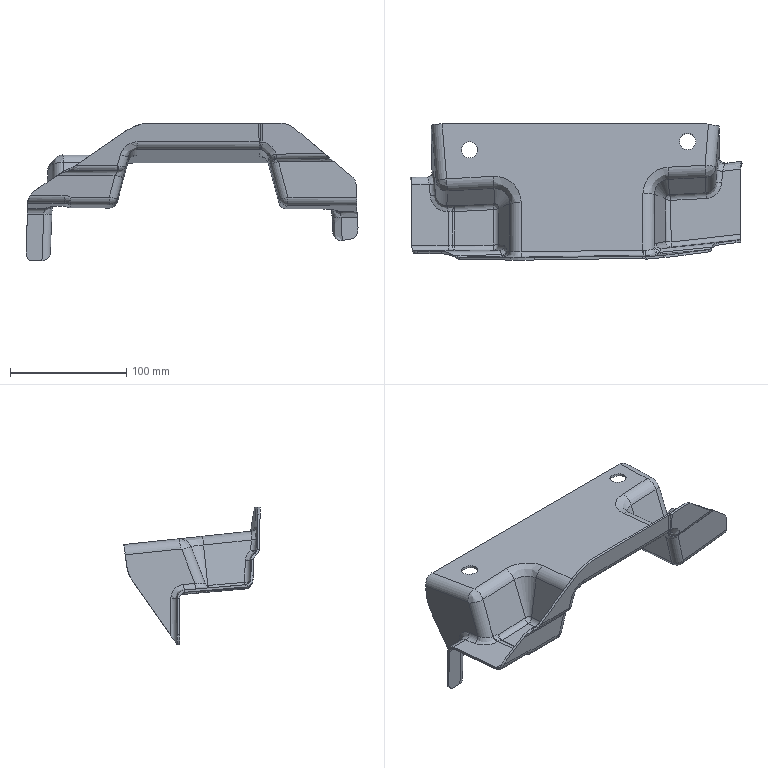Part | 1 solid | 213 faces | box 285.108 x 117.027 x 118.415 mm | volume 99201 mm3 | spline 103 | cylinder 62 | plane 38 | other 6 | sphere 4 | commonest cylinder face diameters 14 x26 10 x20 16 x4 18 x4 20 x4 6 x2